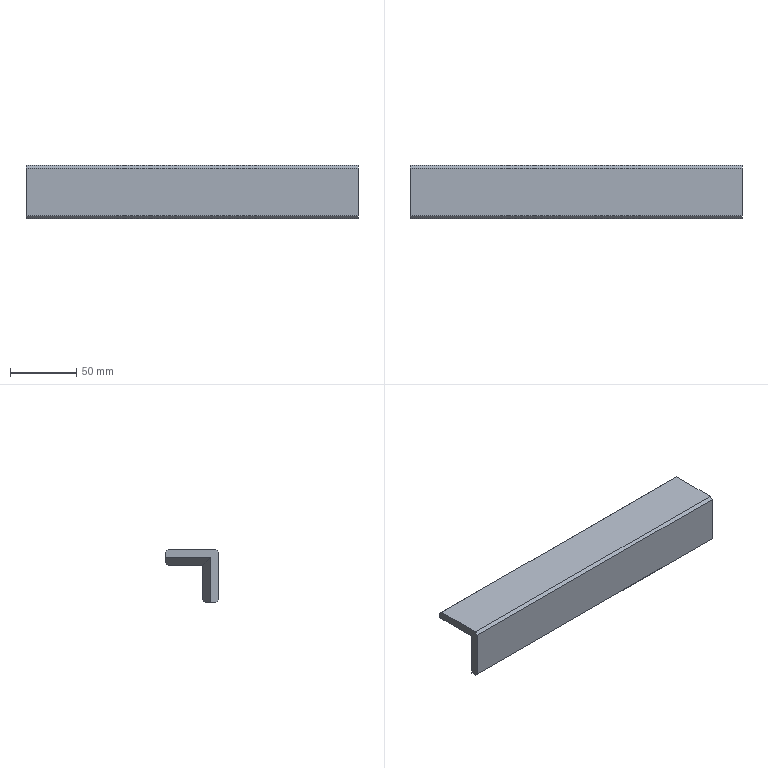CAM job | NX | 3+2 milling | part box 250 x 40 x 40 mm | stock box 255 x 45 x 45 mm
Tools:
number,name,description,diameter,corner_radius,flute_length,length,flutes
9,D10,平底铣刀-粗,10.0,0.0,35.0,75.0,2
10,D10-J,平底铣刀-精,10.0,0.0,35.0,75.0,2
1,D80R0.8飞刀,圆鼻刀-粗,80.0,0.8,50.0,75.0,2
1,D80R0.8飞刀-J,圆鼻刀-精,80.0,0.8,50.0,75.0,2
2,D6倒角刀,倒角刀,6.0,0.0,3.0,25.0,2
Operations:
program,operation,operation_type,tool,method,geometry_group,spindle_rpm,surface_speed,feed_per_tooth,feed_cut,feed_plunge,cut_length_mm,path_length_mm,cut_time_min,machine_time_min
B,底壁铣飞面一刀开粗_COPY,VolumeBased25DMillingOperation,D80R0.8飞刀,分层开粗-切深K-步距G,W-B,2800.0,703.696,0.5357,3000.0,100.0,3223.746,6615.966,1.075,1.414
B,底壁铣飞面一刀精光_COPY,VolumeBased25DMillingOperation,D80R0.8飞刀-J,侧刃精光-切深K-步距G,W-B,4000.0,1005.28,0.125,1000.0,100.0,357.998,453.998,0.358,0.3676
B,型腔铣开粗-中_COPY,CavityMilling,D10,分层开粗-切深K-步距G,W-B,8000.0,251.32,0.25,4000.0,100.0,92147.934,93937.785,23.037,23.311
B,型腔铣开粗-中_COPY_COPY,CavityMilling,D10,分层开粗-切深K-步距G,W-B,8000.0,251.32,0.25,4000.0,100.0,1180.443,1487.681,0.2951,0.3366
B,等高精光往复爬面_COPY_COPY,ZLevelMilling,D10,等高爬面-切深K-步距G,W-B,7000.0,219.911,0.3214,4500.0,100.0,3794.167,3824.808,0.8431,0.8462
B,平面去毛刺6X45L_COPY,SurfaceContour,D6倒角刀,爬面_倒角-切深0-步距G,W-B,6500.0,122.519,0.1154,1500.0,100.0,82.783,531.917,0.0552,0.1001
B,底壁铣倒角_COPY_1,VolumeBased25DMillingOperation,D6倒角刀,爬面_倒角-切深0-步距G,W-B,6500.0,122.522,0.0769,1000.0,100.0,514.32,736.327,0.5143,0.5365
B,C0.3封闭铣廓倒角6X45L_COPY,PlanarMilling,D6倒角刀,爬面_倒角-切深0-步距G,W-B,7000.0,131.0,0.0714,1000.0,100.0,259.2,415.4,0.2592,0.2748
B,底壁铣精光底面-中_COPY,VolumeBased25DMillingOperation,D10-J,精光步距切深关,W-B,7000.0,175.0,0.0536,1500.0,100.0,1526.804,1608.804,1.018,1.026
B,等高精光-中_COPY,ZLevelMilling,D10-J,侧刃精光-切深K-步距G,W-B,8000.0,251.32,0.0625,1000.0,100.0,522.259,896.543,0.5223,0.5597
B,等高精光往复爬面_COPY_1,ZLevelMilling,D10-J,等高爬面-切深K-步距G,W-B,7000.0,219.911,0.3214,4500.0,100.0,25720.518,25811.026,5.716,5.725
A,顶面,FaceMilling,D80R0.8飞刀,侧刃精光-切深K-步距G,W-A,4000.0,1005.31,0.125,1000.0,100.0,344.0,440.0,0.344,0.3536
A,外形粗_2,VolumeBased25DMillingOperation,D10,METHOD,W-A,8000.0,251.327,0.3125,5000.0,80.0,31827.827,31966.627,6.366,6.379
A,等高精光往复爬面_COPY,ZLevelMilling,D10,等高爬面-切深K-步距G,W-A,7000.0,219.911,0.3214,4500.0,100.0,7588.334,7684.024,1.686,1.696
A,仅选体,SurfaceContour,D6倒角刀,METHOD,W-A,8000.0,150.796,0.1875,3000.0,100.0,91.631,532.307,0.0305,0.0746
A,底壁铣倒角_COPY,VolumeBased25DMillingOperation,D6倒角刀,爬面_倒角-切深0-步距G,W-A,6500.0,122.522,0.0769,1000.0,100.0,523.03,770.862,0.523,0.5478
A,外形半精_2,VolumeBased25DMillingOperation,D10-J,METHOD,W-A,8000.0,251.327,0.0625,1000.0,100.0,1849.122,2312.351,1.849,1.895